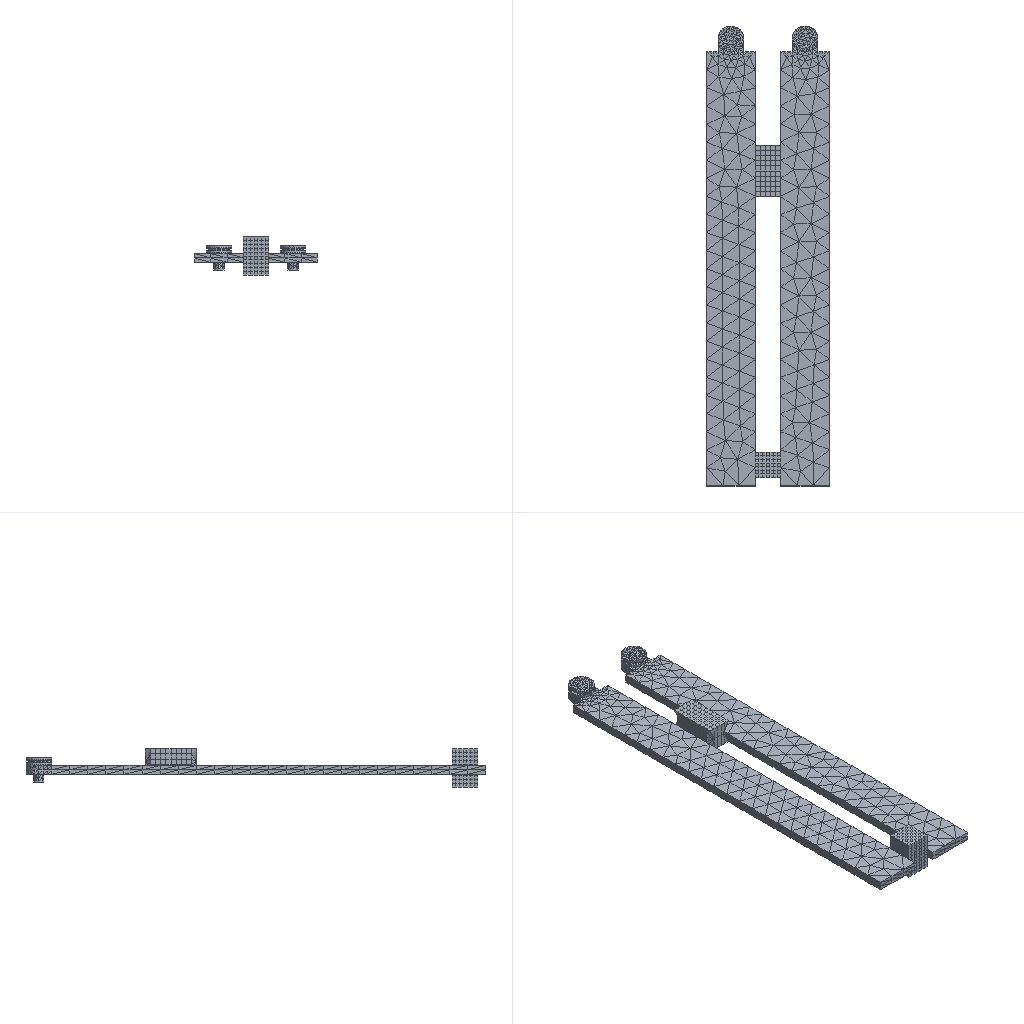Simulation study | abaqus
Set-up summary:
category,name,step,type,value,unit,region
solver,abaqus
solver,version,,,Abaqus/Standard 2020
units,not stated in the deck,,not stated
analysis,deck,,static,static
load_step,Step-1,Step-1,static
load_step,requested,,,1
mesh,nodes,,,3307
mesh,elements,,,7201
element_type,C3D4,,solid,5860
element_type,R3D3,,rigid,108
element_type,R3D4,,rigid,433
element_type,T3D2,,truss,60
element_type,C3D8R,,solid,740
load,load commands in deck,,count,1
bc,support commands in deck,,count,9
material,LV,,in results
material,WIRE,,in results
check,setup vs results,,match,"per instance, exact: element labels, types and connectivity; labels of the nodes the elements use; coordinates of those nodes at SINGLE_PRECISION in 4 of 6 instance(s)"
Abaqus input file, long lists of numbers shortened:
*Heading
** Job name: Job-1 Model name: Model-1
** Generated by: Abaqus/CAE 2020
*Preprint, echo=NO, model=NO, history=NO, contact=NO
**
** PARTS
**
*Part, name=kuai-1
*Node
      1,          10.,           0.,          15.
      2,          10.,  -1.429,          15.
** (702 more lines like these left out)
*Element, type=C3D8R
  1,  89,  90,  98,  97,   1,   2,  10,   9
  2,  90,  91,  99,  98,   2,   3,  11,  10
** (488 more lines like these left out)
*Node
    705,           0.,           0.,          7.5
*Nset, nset=kuai-1-RefPt_, internal
705,
*Nset, nset=Set-2, generate
   1,  704,    1
*Elset, elset=Set-2, generate
   1,  490,    1
** Section: lv
*Solid Section, elset=Set-2, material=lv
,
*End Part
**
*Part, name=kuai-2
*Node
      1,          10.,           0.,          20.
      2,          10.,          -2.,          20.
** (394 more lines like these left out)
*Element, type=C3D8R
  1,  67,  68,  74,  73,   1,   2,   8,   7
  2,  68,  69,  75,  74,   2,   3,   9,   8
** (248 more lines like these left out)
*Node
    397,          10.,           0.,          10.
*Nset, nset=kuai-2-RefPt_, internal
397,
*Nset, nset=Set-2, generate
   1,  396,    1
*Elset, elset=Set-2, generate
   1,  250,    1
** Section: lv
*Solid Section, elset=Set-2, material=lv
,
*End Part
**
*Part, name=wire
*Node
      1,   -2.5,   13.114,           0.
      2,   -2.5,  -86.886,           0.
** (62 more lines like these left out)
*Element, type=T3D2
 1,  1, 11
 2, 11, 12
** (58 more lines like these left out)
*Nset, nset=Set-1, generate
  1,  64,   1
*Elset, elset=Set-1, generate
  1,  60,   1
** Section: wirewire
*Solid Section, elset=Set-1, material=wire
0.2836,
*End Part
**
*Part, name=work-2
*Node
      1,         11.5,       -38.25,           7.
      2,          7.5,       -38.25,           7.
** (830 more lines like these left out)
*Element, type=C3D4
   1, 601, 602, 603, 604
   2, 601, 605, 606, 607
** (2954 more lines like these left out)
*Nset, nset=Set-5, generate
   1,  832,    1
*Elset, elset=Set-5, generate
    1,  2956,     1
** Section: lv
*Solid Section, elset=Set-5, material=lv
,
*End Part
**
*Part, name=work-3
*Node
      1,           0.,        -225.,           0.
      2,          48.,        -225.,           0.
** (483 more lines like these left out)
*Element, type=R3D4
1,  1, 65, 70,  4
2, 65, 66, 69, 70
** (431 more lines like these left out)
*Element, type=R3D3
152, 391, 307, 387
153, 311, 307, 287
** (106 more lines like these left out)
*Node
    486,          48.,       -112.5,           0.
*Nset, nset=work-3-RefPt_, internal
486,
*Elset, elset=work-3, generate
   1,  541,    1
*End Part
**
*Part, name=work-4
*Node
      1,         36.5,       -38.25,           7.
      2,         40.5,       -38.25,           7.
** (821 more lines like these left out)
*Element, type=C3D4
   1, 601, 602, 603, 604
   2, 605, 601, 606, 607
** (2902 more lines like these left out)
*Nset, nset=Set-4, generate
   1,  823,    1
*Elset, elset=Set-4, generate
    1,  2904,     1
** Section: lv
*Solid Section, elset=Set-4, material=lv
,
*End Part
**
**
** ASSEMBLY
**
*Assembly, name=Assembly
**
*Instance, name=work-2-1, part=work-2
*End Instance
**
*Instance, name=work-4-1, part=work-4
*End Instance
**
*Instance, name=work-3-1, part=work-3
*End Instance
**
*Instance, name=kuai-1-1, part=kuai-1
         19.,        -200.,           5.
*End Instance
**
*Instance, name=kuai-2-1, part=kuai-2
         19.,         -80.,          20.
         19.,         -80.,          20., 20.,         -80.,          20., 90.
*End Instance
**
*Instance, name=wire-1, part=wire
   24.,  -113.114,          15.
*End Instance
**
*Nset, nset=Set-6, instance=work-3-1
 486,
*Nset, nset=Set-12, instance=wire-1
  2, 10
*Nset, nset=Set-13, instance=kuai-1-1
   1,   2,   3,   4,   5,   6,   7,   8,   9,  10,  11,  12,  13,  14,  15,  16
  17,  18,  19,  20,  21,  22,  23,  24,  25,  26,  27,  28,  29,  30,  31,  32
** (20 more lines like these left out)
*Elset, elset=Set-13, instance=kuai-1-1
   1,   2,   3,   4,   5,   6,   7,   8,   9,  10,  11,  12,  13,  14,  15,  16
  17,  18,  19,  20,  21,  22,  23,  24,  25,  26,  27,  28,  29,  30,  31,  32
** (15 more lines like these left out)
*Nset, nset=Set-14, instance=kuai-2-1
   1,   2,   3,   4,   5,   6,   7,   8,   9,  10,  11,  12,  13,  14,  15,  16
  17,  18,  19,  20,  21,  22,  23,  24,  25,  26,  27,  28,  29,  30,  31,  32
** (12 more lines like these left out)
*Elset, elset=Set-14, instance=kuai-2-1
   1,   2,   3,   4,   5,   6,   7,   8,   9,  10,  11,  12,  13,  14,  15,  16
  17,  18,  19,  20,  21,  22,  23,  24,  25,  26,  27,  28,  29,  30,  31,  32
** (8 more lines like these left out)
*Nset, nset=m_Set-8, instance=wire-1
  3,  4, 30, 31
*Elset, elset=m_Set-8, instance=wire-1, generate
 21,  23,   1
*Nset, nset=m_Set-9, instance=wire-1
  6,  7, 38, 39
*Elset, elset=m_Set-9, instance=wire-1, generate
 31,  33,   1
*Nset, nset=m_Set-10, instance=wire-1
 5, 8
*Nset, nset=m_Set-11, instance=wire-1
 1, 9
*Nset, nset=m_Set-15, instance=wire-1
 3,
*Nset, nset=m_Set-16, instance=wire-1
 6,
*Elset, elset=_s_Surf-1_S1, internal, instance=work-2-1
  299, 1980
*Elset, elset=_s_Surf-1_S4, internal, instance=work-2-1
  625, 1752, 1893, 2233
*Elset, elset=_s_Surf-1_S3, internal, instance=work-2-1
  805, 1579, 1586, 1627, 1654, 1759, 1777, 1778, 1822, 1856, 1872, 1874, 1896, 1915, 1952, 1955
 1956, 1969, 1979, 1984, 1991, 1998, 1999, 2002, 2004, 2009, 2016, 2021, 2028, 2034, 2042, 2050
** (3 more lines like these left out)
*Elset, elset=_s_Surf-1_S2, internal, instance=work-2-1
 1873, 1964, 2047, 2091
*Surface, type=ELEMENT, name=s_Surf-1
_s_Surf-1_S1, S1
_s_Surf-1_S4, S4
_s_Surf-1_S2, S2
_s_Surf-1_S3, S3
*Elset, elset=_s_Surf-2_S3, internal, instance=work-4-1
  390,  897, 1146, 1263, 1308, 1385, 1445, 1569, 1617, 1745, 1809, 1820, 1856, 1858, 1866, 1918
 1923, 1930, 1931, 1948, 1955, 1962, 1968, 1974, 1975, 1979, 1980, 1992, 1998, 2001, 2014, 2019
** (3 more lines like these left out)
*Elset, elset=_s_Surf-2_S1, internal, instance=work-4-1
 1208, 2158, 2708
*Elset, elset=_s_Surf-2_S4, internal, instance=work-4-1
 1270, 1942, 2055, 2082, 2397
*Elset, elset=_s_Surf-2_S2, internal, instance=work-4-1
 1843, 1967, 2056
*Surface, type=ELEMENT, name=s_Surf-2
_s_Surf-2_S3, S3
_s_Surf-2_S1, S1
_s_Surf-2_S4, S4
_s_Surf-2_S2, S2
*Elset, elset=_s_Surf-3_S5, internal, instance=kuai-2-1
  46,  47,  48,  49,  50,  96,  97,  98,  99, 100, 146, 147, 148, 149, 150, 196
 197, 198, 199, 200, 246, 247, 248, 249, 250
*Surface, type=ELEMENT, name=s_Surf-3
_s_Surf-3_S5, S5
*Elset, elset=_s_Surf-4_S3, internal, instance=kuai-2-1
   1,   2,   3,   4,   5,  51,  52,  53,  54,  55, 101, 102, 103, 104, 105, 151
 152, 153, 154, 155, 201, 202, 203, 204, 205
*Surface, type=ELEMENT, name=s_Surf-4
_s_Surf-4_S3, S3
*Surface, type=NODE, name=m_Set-15_CNS_, internal
m_Set-15, 1.
*Surface, type=NODE, name=m_Set-16_CNS_, internal
m_Set-16, 1.
*Surface, type=NODE, name=m_Set-10_CNS_, internal
m_Set-10, 1.
*Surface, type=NODE, name=m_Set-11_CNS_, internal
m_Set-11, 1.
*Rigid Body, ref node=work-3-1.work-3-RefPt_, elset=work-3-1.work-3
** Constraint: Constraint-1
*Tie, name=Constraint-1, adjust=yes
s_Surf-1, m_Set-15_CNS_
** Constraint: Constraint-2
*Tie, name=Constraint-2, adjust=yes
s_Surf-2, m_Set-16_CNS_
** Constraint: Constraint-3
*Tie, name=Constraint-3, adjust=yes
s_Surf-3, m_Set-10_CNS_
** Constraint: Constraint-4
*Tie, name=Constraint-4, adjust=yes
s_Surf-4, m_Set-11_CNS_
*Elset, elset=__Int-1_gcs0_6_S1, internal, instance=work-2-1
  299, 1980
*Elset, elset=__Int-1_gcs0_6_S4, internal, instance=work-2-1
  625, 1752, 1893, 2233
*Elset, elset=__Int-1_gcs0_6_S3, internal, instance=work-2-1
  805, 1579, 1586, 1627, 1654, 1759, 1777, 1778, 1822, 1856, 1872, 1874, 1896, 1915, 1952, 1955
 1956, 1969, 1979, 1984, 1991, 1998, 1999, 2002, 2004, 2009, 2016, 2021, 2028, 2034, 2042, 2050
** (3 more lines like these left out)
*Elset, elset=__Int-1_gcs0_6_S2, internal, instance=work-2-1
 1873, 1964, 2047, 2091
*Surface, type=ELEMENT, name=_Int-1_gcs0_6, internal
__Int-1_gcs0_6_S1, S1
__Int-1_gcs0_6_S4, S4
__Int-1_gcs0_6_S2, S2
__Int-1_gcs0_6_S3, S3
*Elset, elset=__Int-1_gcs0_12_S3, internal, instance=work-2-1
  357, 1003, 1286, 1420, 1714, 1774, 2281, 2284, 2562, 2574
*Elset, elset=__Int-1_gcs0_12_S1, internal, instance=work-2-1
  886, 1575
*Elset, elset=__Int-1_gcs0_12_S4, internal, instance=work-2-1
 1135, 1580, 1905, 1975, 2329, 2551
*Surface, type=ELEMENT, name=_Int-1_gcs0_12, internal
__Int-1_gcs0_12_S3, S3
__Int-1_gcs0_12_S1, S1
__Int-1_gcs0_12_S4, S4
*Elset, elset=__Int-1_gcs0_22_S1, internal, instance=work-2-1
  181,  333,  527,  610, 1193, 1628, 1679, 1858, 1916, 1986, 2104, 2115, 2193, 2306, 2397, 2398
 2399, 2465, 2508, 2548, 2737, 2751, 2777, 2863, 2903
*Elset, elset=__Int-1_gcs0_22_S3, internal, instance=work-2-1
  346,  423,  439,  444,  568,  586,  591,  592,  617,  631,  652,  669,  690,  716,  743,  760
  843,  850,  867,  884,  941,  961, 1058, 1069, 1128, 1152, 1169, 1170, 1278, 1313, 1391, 1393
** (2 more lines like these left out)
*Elset, elset=__Int-1_gcs0_22_S4, internal, instance=work-2-1
  354,  907, 1092, 1377, 2057, 2212, 2374, 2376, 2408, 2452, 2692, 2738, 2803, 2827, 2829, 2867
*Elset, elset=__Int-1_gcs0_22_S2, internal, instance=work-2-1
  366, 1990, 2011, 2068, 2114, 2142, 2280, 2439, 2483, 2511, 2512, 2517, 2518, 2533, 2586, 2588
 2593, 2606, 2607, 2635, 2779, 2804
*Surface, type=ELEMENT, name=_Int-1_gcs0_22, internal
__Int-1_gcs0_22_S1, S1
__Int-1_gcs0_22_S3, S3
__Int-1_gcs0_22_S4, S4
__Int-1_gcs0_22_S2, S2
*Elset, elset=__Int-1_gcs0_23_S2, internal, instance=work-2-1
  167,  644, 1503, 1833
*Elset, elset=__Int-1_gcs0_23_S1, internal, instance=work-2-1
  612,  640, 1750
*Elset, elset=__Int-1_gcs0_23_S3, internal, instance=work-2-1
  641,  650,  794,  842, 1141, 1143, 1315, 1498, 1703, 1724, 1784, 1786, 1796, 1800, 1802, 1807
 1810, 1818, 1819, 1907, 1970, 2182, 2346
*Elset, elset=__Int-1_gcs0_23_S4, internal, instance=work-2-1
  642, 1767
*Surface, type=ELEMENT, name=_Int-1_gcs0_23, internal
__Int-1_gcs0_23_S2, S2
__Int-1_gcs0_23_S1, S1
__Int-1_gcs0_23_S4, S4
__Int-1_gcs0_23_S3, S3
*Elset, elset=__Int-1_gcs0_24_S3, internal, instance=work-2-1
  837, 1407, 1445, 1783, 1844, 1849, 1918
*Elset, elset=__Int-1_gcs0_24_S1, internal, instance=work-2-1
 1447, 1450, 1864
*Elset, elset=__Int-1_gcs0_24_S4, internal, instance=work-2-1
 1831, 1876, 1888, 1912
*Elset, elset=__Int-1_gcs0_24_S2, internal, instance=work-2-1
 1935, 2648
*Surface, type=ELEMENT, name=_Int-1_gcs0_24, internal
__Int-1_gcs0_24_S3, S3
__Int-1_gcs0_24_S1, S1
__Int-1_gcs0_24_S4, S4
__Int-1_gcs0_24_S2, S2
*Elset, elset=__Int-1_gcs0_30_S3, internal, instance=work-4-1
  390,  897, 1146, 1263, 1308, 1385, 1445, 1569, 1617, 1745, 1809, 1820, 1856, 1858, 1866, 1918
 1923, 1930, 1931, 1948, 1955, 1962, 1968, 1974, 1975, 1979, 1980, 1992, 1998, 2001, 2014, 2019
** (3 more lines like these left out)
*Elset, elset=__Int-1_gcs0_30_S1, internal, instance=work-4-1
 1208, 2158, 2708
*Elset, elset=__Int-1_gcs0_30_S4, internal, instance=work-4-1
 1270, 1942, 2055, 2082, 2397
*Elset, elset=__Int-1_gcs0_30_S2, internal, instance=work-4-1
 1843, 1967, 2056
*Surface, type=ELEMENT, name=_Int-1_gcs0_30, internal
__Int-1_gcs0_30_S3, S3
__Int-1_gcs0_30_S1, S1
__Int-1_gcs0_30_S4, S4
__Int-1_gcs0_30_S2, S2
*Elset, elset=__Int-1_gcs0_36_S3, internal, instance=work-4-1
  297,  769,  801,  802,  907,  918, 1899, 2351, 2353, 2368, 2371, 2821
*Elset, elset=__Int-1_gcs0_36_S1, internal, instance=work-4-1
  790, 1002, 2783
*Elset, elset=__Int-1_gcs0_36_S2, internal, instance=work-4-1
  826, 1468
*Elset, elset=__Int-1_gcs0_36_S4, internal, instance=work-4-1
 2363,
*Surface, type=ELEMENT, name=_Int-1_gcs0_36, internal
__Int-1_gcs0_36_S3, S3
__Int-1_gcs0_36_S1, S1
__Int-1_gcs0_36_S2, S2
__Int-1_gcs0_36_S4, S4
*Elset, elset=__Int-1_gcs0_46_S4, internal, instance=work-4-1
   41,  109,  278,  688,  782,  845, 1217, 1236, 1278, 1758, 1848, 2279, 2297, 2409, 2483, 2505
 2579, 2745, 2749, 2813, 2864, 2877, 2887, 2894
*Elset, elset=__Int-1_gcs0_46_S1, internal, instance=work-4-1
   73,  245,  847,  932,  951, 1055, 1255, 1531, 1778, 1912, 1977, 1995, 2260, 2432, 2727, 2752
 2765, 2806, 2882, 2898
*Elset, elset=__Int-1_gcs0_46_S2, internal, instance=work-4-1
  244,  467,  504, 1476, 1588, 1763, 1883, 1901, 2552, 2575, 2652, 2667, 2674, 2770, 2803, 2811
 2841, 2880
*Elset, elset=__Int-1_gcs0_46_S3, internal, instance=work-4-1
  441,  526,  528,  563,  582,  585,  606,  616,  636,  662,  868,  887,  999, 1018, 1045, 1113
 1140, 1191, 1254, 1277, 1282, 1283, 1284, 1294, 1328, 1386, 1402, 1430, 1432, 1482, 1484, 1490
** (2 more lines like these left out)
*Surface, type=ELEMENT, name=_Int-1_gcs0_46, internal
__Int-1_gcs0_46_S4, S4
__Int-1_gcs0_46_S1, S1
__Int-1_gcs0_46_S2, S2
__Int-1_gcs0_46_S3, S3
*Elset, elset=__Int-1_gcs0_47_S3, internal, instance=work-4-1
   97,  641, 1336, 1505, 1586, 1618, 1627, 1688, 1712, 1720, 1723, 1727, 1755, 1762, 1773, 1776
 1781, 1792, 1793, 1796, 1875, 2737, 2757
*Elset, elset=__Int-1_gcs0_47_S4, internal, instance=work-4-1
  794, 1700, 1754, 1800, 2641
*Elset, elset=__Int-1_gcs0_47_S2, internal, instance=work-4-1
 1333, 1593, 1698, 1748
*Surface, type=ELEMENT, name=_Int-1_gcs0_47, internal
__Int-1_gcs0_47_S3, S3
__Int-1_gcs0_47_S4, S4
__Int-1_gcs0_47_S2, S2
*Elset, elset=__Int-1_gcs0_48_S1, internal, instance=work-4-1
  127,  832, 1114, 2161
*Elset, elset=__Int-1_gcs0_48_S2, internal, instance=work-4-1
  684, 1849
*Elset, elset=__Int-1_gcs0_48_S3, internal, instance=work-4-1
  834, 1116, 1156, 1876, 1898, 1911, 1915, 1984, 2156
*Elset, elset=__Int-1_gcs0_48_S4, internal, instance=work-4-1
 1832,
*Surface, type=ELEMENT, name=_Int-1_gcs0_48, internal
__Int-1_gcs0_48_S1, S1
__Int-1_gcs0_48_S2, S2
__Int-1_gcs0_48_S4, S4
__Int-1_gcs0_48_S3, S3
*Elset, elset=__Int-1_gcs0_55_SPOS, internal, instance=work-3-1, generate
 89,  95,   1
*Surface, type=ELEMENT, name=_Int-1_gcs0_55, internal
__Int-1_gcs0_55_SPOS, SPOS
*Elset, elset=__Int-1_gcs0_57_SPOS, internal, instance=work-3-1, generate
  96,  102,    1
*Surface, type=ELEMENT, name=_Int-1_gcs0_57, internal
__Int-1_gcs0_57_SPOS, SPOS
*Elset, elset=__Int-1_gcs0_80_SPOS, internal, instance=work-3-1, generate
 124,  131,    1
*Surface, type=ELEMENT, name=_Int-1_gcs0_80, internal
__Int-1_gcs0_80_SPOS, SPOS
*Elset, elset=__Int-1_gcs0_81_SPOS, internal, instance=work-3-1, generate
 132,  139,    1
*Surface, type=ELEMENT, name=_Int-1_gcs0_81, internal
__Int-1_gcs0_81_SPOS, SPOS
*Elset, elset=__Int-1_gcs0_82_SPOS, internal, instance=work-3-1, generate
 140,  145,    1
*Surface, type=ELEMENT, name=_Int-1_gcs0_82, internal
__Int-1_gcs0_82_SPOS, SPOS
*Elset, elset=__Int-1_gcs0_83_SPOS, internal, instance=work-3-1, generate
 146,  151,    1
*Surface, type=ELEMENT, name=_Int-1_gcs0_83, internal
__Int-1_gcs0_83_SPOS, SPOS
*Elset, elset=__Int-1_gcs0_90_SNEG, internal, instance=work-3-1, generate
 89,  95,   1
*Surface, type=ELEMENT, name=_Int-1_gcs0_90, internal
__Int-1_gcs0_90_SNEG, SNEG
*Elset, elset=__Int-1_gcs0_92_SNEG, internal, instance=work-3-1, generate
  96,  102,    1
*Surface, type=ELEMENT, name=_Int-1_gcs0_92, internal
__Int-1_gcs0_92_SNEG, SNEG
*Elset, elset=__Int-1_gcs0_115_SNEG, internal, instance=work-3-1, generate
 124,  131,    1
*Surface, type=ELEMENT, name=_Int-1_gcs0_115, internal
__Int-1_gcs0_115_SNEG, SNEG
*Elset, elset=__Int-1_gcs0_116_SNEG, internal, instance=work-3-1, generate
 132,  139,    1
*Surface, type=ELEMENT, name=_Int-1_gcs0_116, internal
__Int-1_gcs0_116_SNEG, SNEG
*Elset, elset=__Int-1_gcs0_117_SNEG, internal, instance=work-3-1, generate
 140,  145,    1
*Surface, type=ELEMENT, name=_Int-1_gcs0_117, internal
__Int-1_gcs0_117_SNEG, SNEG
*Elset, elset=__Int-1_gcs0_118_SNEG, internal, instance=work-3-1, generate
 146,  151,    1
*Surface, type=ELEMENT, name=_Int-1_gcs0_118, internal
__Int-1_gcs0_118_SNEG, SNEG
*End Assembly
*Amplitude, name=Amp-1
             0.,              0.,              1.,              1.
**
** MATERIALS
**
*Material, name=lv
*Density
 2.7e-09,
*Elastic
78000., 0.35
*Material, name=wire
*Density
 7.8e-09,
*Elastic
1700., 0.4
**
** INTERACTION PROPERTIES
**
*Surface Interaction, name=IntProp-1
1.,
*Friction
0.,
*Surface Behavior, pressure-overclosure=HARD
**
** INTERACTIONS
**
** Interaction: Int-1
*Contact
*Contact Inclusions, ALL EXTERIOR
*Contact Property Assignment
 ,  , IntProp-1
*Surface Property Assignment, property=GEOMETRIC CORRECTION
_Int-1_gcs0_6, Circumferential, 9.5, -38.25, 15.5,  9.5, -38.25, 14.5
_Int-1_gcs0_12, Circumferential, 9.5, -38.25, 10.5,  9.5, -38.25, 9.5
_Int-1_gcs0_22, Circumferential, 9.5, -38.25, 16.5,  9.5, -38.25, 15.5
_Int-1_gcs0_23, Circumferential, 9.5, -38.25, 7.,  9.5, -38.25, 8.
_Int-1_gcs0_24, Circumferential, 10.25, -42.579, 15.,  9.25, -42.579, 15.
_Int-1_gcs0_30, Circumferential, 38.5, -38.25, 15.5,  38.5, -38.25, 14.5
_Int-1_gcs0_36, Circumferential, 38.5, -38.25, 10.5,  38.5, -38.25, 9.5
_Int-1_gcs0_46, Circumferential, 38.5, -38.25, 16.5,  38.5, -38.25, 15.5
_Int-1_gcs0_47, Circumferential, 38.5, -38.25, 7.,  38.5, -38.25, 8.
_Int-1_gcs0_48, Circumferential, 37.75, -42.579, 15.,  38.75, -42.579, 15.
_Int-1_gcs0_55, Circumferential, 38.5, -38.25, 10.,  38.5, -38.25, 9.
_Int-1_gcs0_57, Circumferential, 9.5, -38.25, 10.,  9.5, -38.25, 9.
_Int-1_gcs0_80, Circumferential, 38.5, -38.25, 8.,  38.5, -38.25, 7.
_Int-1_gcs0_81, Circumferential, 9.5, -38.25, 8.,  9.5, -38.25, 7.
_Int-1_gcs0_82, Circumferential, 21.5, -52.5, 15.,  21.5, -51.5, 15.
_Int-1_gcs0_83, Circumferential, 26.5, -52.5, 15.,  26.5, -51.5, 15.
_Int-1_gcs0_90, Circumferential, 38.5, -38.25, 10.,  38.5, -38.25, 9.
_Int-1_gcs0_92, Circumferential, 9.5, -38.25, 10.,  9.5, -38.25, 9.
_Int-1_gcs0_115, Circumferential, 38.5, -38.25, 8.,  38.5, -38.25, 7.
_Int-1_gcs0_116, Circumferential, 9.5, -38.25, 8.,  9.5, -38.25, 7.
_Int-1_gcs0_117, Circumferential, 21.5, -52.5, 15.,  21.5, -51.5, 15.
_Int-1_gcs0_118, Circumferential, 26.5, -52.5, 15.,  26.5, -51.5, 15.
** ----------------------------------------------------------------
**
** STEP: Step-1
**
*Step, name=Step-1, nlgeom=YES, inc=1000
*Static, stabilize=0.0002, allsdtol=0.05, continue=NO
0.001, 1., 1e-05, 1.
**
** BOUNDARY CONDITIONS
**
** Name: BC-1 Type: 对称/反对称/完全固定
*Boundary
Set-13, ENCASTRE
** Name: BC-2 Type: 对称/反对称/完全固定
*Boundary
Set-6, ENCASTRE
** Name: BC-3 Type: 位移/转角
*Boundary, amplitude=Amp-1
Set-14, 1, 1
Set-14, 2, 2, -10.
Set-14, 3, 3
Set-14, 4, 4
Set-14, 5, 5
Set-14, 6, 6
** Name: BC-4 Type: 对称/反对称/完全固定
*Boundary
Set-12, ENCASTRE
**
** OUTPUT REQUESTS
**
*Restart, write, frequency=0
**
** FIELD OUTPUT: F-Output-1
**
*Output, field
*Node Output
CF, RF, RT, TF, U, V
*Element Output, directions=YES
E, LE, MISES, PE, PEEQ, PEMAG, S, SF
*Contact Output
CDISP, CSTRESS
**
** HISTORY OUTPUT: H-Output-1
**
*Output, history, variable=PRESELECT
*End Step
Results summary:
result,step,,partial,increments=0 time=0.0/1.0
result,analysis,,,static
result,last_loadstep,,,1
result,primary field,,,U
result,reaction total,,FX,0.0,model units
result,reaction total,,FY,0.0,model units
result,reaction total,,FZ,0.0,model units